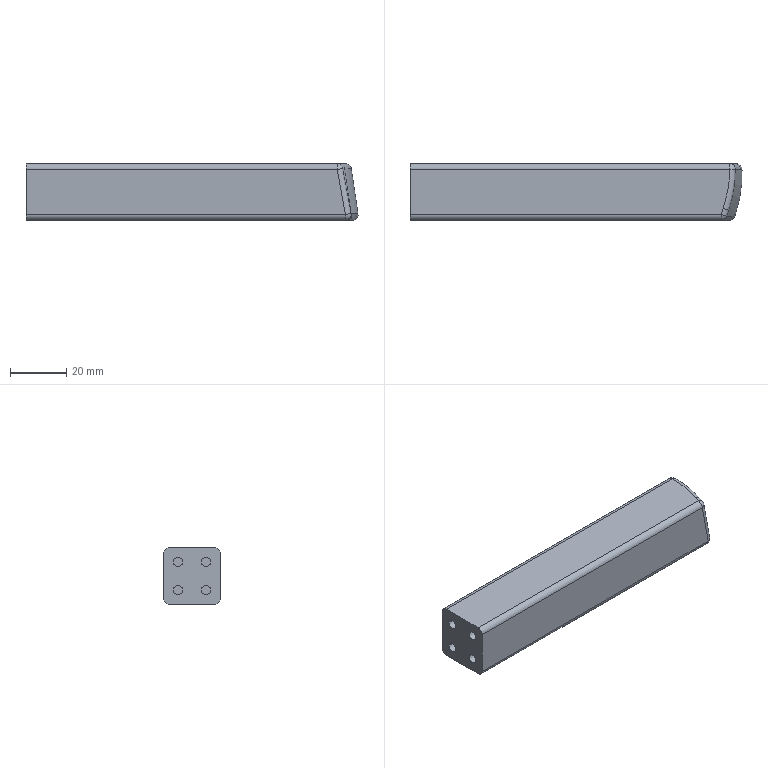NC program | NX | posted with a generic post | part box 117.695 x 20 x 20.003 mm
Whole program:
N10 G17 G21 G94 G90
(DRILLING_COPY , TOOL : D4A45)
N12 T02 M6
N14 G54
N16 G17 G0 G90 X-5. Y-5. B0. C0. S5000 M3
N18 G43 Z30. H2
N20 G94 G81 G98 Z-1. F250. R3.
N22 Y5.
N24 X5.
N26 Y-5.
N28 G80
N30 G0 X5. Y-5. Z30.
N32 M5
(DRILLING_COPY_COPY , TOOL : 3.3ZT)
N34 T12 M6
N36 G54
N38 G17 G0 G90 X-5. Y-5. B0. C0. S1910 M3
N40 G43 Z30. H12
N42 G94 G83 G98 Z-12. F180. Q2. R3.
N44 Y5.
N46 X5.
N48 Y-5.
N50 G80
N52 G0 X5. Y-5. Z30.
N54 M5
N56 M2